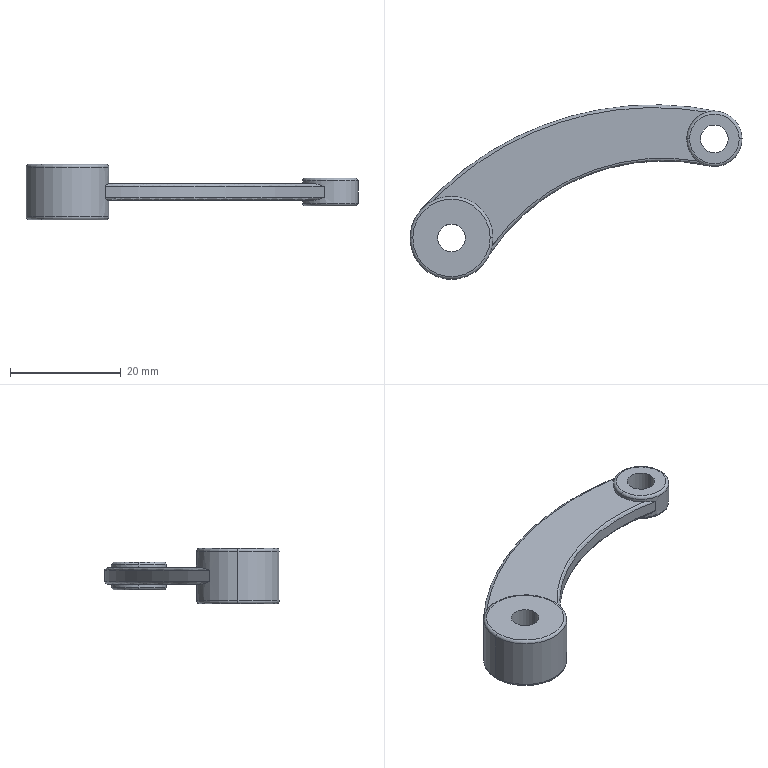Part | SolidWorks | features Fillet 2, ICE 2, Extrusion 1, MirrorPattern 1 | 1 solid | 28 faces | box 60.037 x 31.564 x 10 mm | volume 3346 mm3 | torus 12 | cylinder 10 | plane 6 | commonest cylinder face diameters 5 x4 10 x2 15 x2 75.265 x1 112.752 x1
STEP:
#1=CARTESIAN_POINT('',(-7.5,0.,4.5));
#2=VERTEX_POINT('',#1);
#3=CARTESIAN_POINT('',(7.5,0.,4.5));
#4=VERTEX_POINT('',#3);
#5=CARTESIAN_POINT('',(0.,0.,4.5));
#6=DIRECTION('',(0.,0.,-1.));
#7=DIRECTION('',(1.,0.,0.));
#8=AXIS2_PLACEMENT_3D('',#5,#6,#7);
#9=CIRCLE('',#8,7.5);
#10=EDGE_CURVE('',#2,#4,#9,.T.);
#11=ORIENTED_EDGE('',*,*,#10,.F.);
#12=CARTESIAN_POINT('',(-7.,0.,5.));
#13=VERTEX_POINT('',#12);
#14=CARTESIAN_POINT('',(-7.,0.,4.5));
#15=DIRECTION('',(0.,1.,0.));
#16=DIRECTION('',(-1.,0.,0.));
#17=AXIS2_PLACEMENT_3D('',#14,#15,#16);
#18=CIRCLE('',#17,0.5);
#19=EDGE_CURVE('',#2,#13,#18,.T.);
#20=ORIENTED_EDGE('',*,*,#19,.T.);
#21=CARTESIAN_POINT('',(7.,0.,5.));
#22=VERTEX_POINT('',#21);
#23=CARTESIAN_POINT('',(0.,0.,5.));
#24=DIRECTION('',(0.,0.,1.));
#25=DIRECTION('',(1.,0.,0.));
#26=AXIS2_PLACEMENT_3D('',#23,#24,#25);
#27=CIRCLE('',#26,7.);
#28=EDGE_CURVE('',#22,#13,#27,.T.);
#29=ORIENTED_EDGE('',*,*,#28,.F.);
#30=CARTESIAN_POINT('',(7.,0.,4.5));
#31=DIRECTION('',(0.,-1.,0.));
#32=DIRECTION('',(0.,0.,-1.));
#33=AXIS2_PLACEMENT_3D('',#30,#31,#32);
#34=CIRCLE('',#33,0.5);
#35=EDGE_CURVE('',#4,#22,#34,.T.);
#36=ORIENTED_EDGE('',*,*,#35,.F.);
#37=EDGE_LOOP('',(#11,#20,#29,#36));
#38=FACE_OUTER_BOUND('',#37,.T.);
#39=CARTESIAN_POINT('',(0.,0.,4.5));
#40=DIRECTION('',(0.,0.,1.));
#41=DIRECTION('',(1.,0.,0.));
#42=AXIS2_PLACEMENT_3D('',#39,#40,#41);
#43=TOROIDAL_SURFACE('',#42,7.,0.5);
#44=ADVANCED_FACE('',(#38),#43,.T.);
#45=CARTESIAN_POINT('',(42.537,17.903,2.));
#46=VERTEX_POINT('',#45);
#47=CARTESIAN_POINT('',(52.537,17.903,2.));
#48=VERTEX_POINT('',#47);
#49=CARTESIAN_POINT('',(47.537,17.903,2.));
#50=DIRECTION('',(0.,0.,-1.));
#51=DIRECTION('',(1.,0.,0.));
#52=AXIS2_PLACEMENT_3D('',#49,#50,#51);
#53=CIRCLE('',#52,5.);
#54=EDGE_CURVE('',#46,#48,#53,.T.);
#55=ORIENTED_EDGE('',*,*,#54,.F.);
#56=CARTESIAN_POINT('',(43.037,17.903,2.5));
#57=VERTEX_POINT('',#56);
#58=CARTESIAN_POINT('',(43.037,17.903,2.));
#59=DIRECTION('',(0.,1.,0.));
#60=DIRECTION('',(-1.,0.,0.));
#61=AXIS2_PLACEMENT_3D('',#58,#59,#60);
#62=CIRCLE('',#61,0.5);
#63=EDGE_CURVE('',#46,#57,#62,.T.);
#64=ORIENTED_EDGE('',*,*,#63,.T.);
#65=CARTESIAN_POINT('',(52.037,17.903,2.5));
#66=VERTEX_POINT('',#65);
#67=CARTESIAN_POINT('',(47.537,17.903,2.5));
#68=DIRECTION('',(0.,0.,1.));
#69=DIRECTION('',(1.,0.,0.));
#70=AXIS2_PLACEMENT_3D('',#67,#68,#69);
#71=CIRCLE('',#70,4.5);
#72=EDGE_CURVE('',#66,#57,#71,.T.);
#73=ORIENTED_EDGE('',*,*,#72,.F.);
#74=CARTESIAN_POINT('',(52.037,17.903,2.));
#75=DIRECTION('',(0.,-1.,0.));
#76=DIRECTION('',(0.,0.,-1.));
#77=AXIS2_PLACEMENT_3D('',#74,#75,#76);
#78=CIRCLE('',#77,0.5);
#79=EDGE_CURVE('',#48,#66,#78,.T.);
#80=ORIENTED_EDGE('',*,*,#79,.F.);
#81=EDGE_LOOP('',(#55,#64,#73,#80));
#82=FACE_OUTER_BOUND('',#81,.T.);
#83=CARTESIAN_POINT('',(47.537,17.903,2.));
#84=DIRECTION('',(0.,0.,1.));
#85=DIRECTION('',(1.,0.,0.));
#86=AXIS2_PLACEMENT_3D('',#83,#84,#85);
#87=TOROIDAL_SURFACE('',#86,4.5,0.5);
#88=ADVANCED_FACE('',(#82),#87,.T.);
#89=CARTESIAN_POINT('',(52.537,17.903,-2.));
#90=VERTEX_POINT('',#89);
#91=CARTESIAN_POINT('',(42.537,17.903,-2.));
#92=VERTEX_POINT('',#91);
#93=CARTESIAN_POINT('',(47.537,17.903,-2.));
#94=DIRECTION('',(0.,0.,1.));
#95=DIRECTION('',(-1.,0.,0.));
#96=AXIS2_PLACEMENT_3D('',#93,#94,#95);
#97=CIRCLE('',#96,5.);
#98=EDGE_CURVE('',#90,#92,#97,.T.);
#99=ORIENTED_EDGE('',*,*,#98,.F.);
#100=CARTESIAN_POINT('',(52.037,17.903,-2.5));
#101=VERTEX_POINT('',#100);
#102=CARTESIAN_POINT('',(52.037,17.903,-2.));
#103=DIRECTION('',(0.,1.,0.));
#104=DIRECTION('',(-1.,0.,0.));
#105=AXIS2_PLACEMENT_3D('',#102,#103,#104);
#106=CIRCLE('',#105,0.5);
#107=EDGE_CURVE('',#90,#101,#106,.T.);
#108=ORIENTED_EDGE('',*,*,#107,.T.);
#109=CARTESIAN_POINT('',(43.037,17.903,-2.5));
#110=VERTEX_POINT('',#109);
#111=CARTESIAN_POINT('',(47.537,17.903,-2.5));
#112=DIRECTION('',(0.,0.,-1.));
#113=DIRECTION('',(-1.,0.,0.));
#114=AXIS2_PLACEMENT_3D('',#111,#112,#113);
#115=CIRCLE('',#114,4.5);
#116=EDGE_CURVE('',#110,#101,#115,.T.);
#117=ORIENTED_EDGE('',*,*,#116,.F.);
#118=CARTESIAN_POINT('',(43.037,17.903,-2.));
#119=DIRECTION('',(0.,-1.,0.));
#120=DIRECTION('',(0.,0.,-1.));
#121=AXIS2_PLACEMENT_3D('',#118,#119,#120);
#122=CIRCLE('',#121,0.5);
#123=EDGE_CURVE('',#92,#110,#122,.T.);
#124=ORIENTED_EDGE('',*,*,#123,.F.);
#125=EDGE_LOOP('',(#99,#108,#117,#124));
#126=FACE_OUTER_BOUND('',#125,.T.);
#127=CARTESIAN_POINT('',(47.537,17.903,-2.));
#128=DIRECTION('',(0.,0.,-1.));
#129=DIRECTION('',(-1.,0.,0.));
#130=AXIS2_PLACEMENT_3D('',#127,#128,#129);
#131=TOROIDAL_SURFACE('',#130,4.5,0.5);
#132=ADVANCED_FACE('',(#126),#131,.T.);
#133=CARTESIAN_POINT('',(-7.,0.,-5.));
#134=VERTEX_POINT('',#133);
#135=CARTESIAN_POINT('',(7.,0.,-5.));
#136=VERTEX_POINT('',#135);
#137=CARTESIAN_POINT('',(0.,0.,-5.));
#138=DIRECTION('',(0.,0.,-1.));
#139=DIRECTION('',(1.,0.,0.));
#140=AXIS2_PLACEMENT_3D('',#137,#138,#139);
#141=CIRCLE('',#140,7.);
#142=EDGE_CURVE('',#134,#136,#141,.T.);
#143=ORIENTED_EDGE('',*,*,#142,.F.);
#144=CARTESIAN_POINT('',(-7.5,0.,-4.5));
#145=VERTEX_POINT('',#144);
#146=CARTESIAN_POINT('',(-7.,0.,-4.5));
#147=DIRECTION('',(0.,1.,0.));
#148=DIRECTION('',(-1.,0.,0.));
#149=AXIS2_PLACEMENT_3D('',#146,#147,#148);
#150=CIRCLE('',#149,0.5);
#151=EDGE_CURVE('',#134,#145,#150,.T.);
#152=ORIENTED_EDGE('',*,*,#151,.T.);
#153=CARTESIAN_POINT('',(7.5,0.,-4.5));
#154=VERTEX_POINT('',#153);
#155=CARTESIAN_POINT('',(0.,0.,-4.5));
#156=DIRECTION('',(0.,0.,1.));
#157=DIRECTION('',(1.,0.,0.));
#158=AXIS2_PLACEMENT_3D('',#155,#156,#157);
#159=CIRCLE('',#158,7.5);
#160=EDGE_CURVE('',#154,#145,#159,.T.);
#161=ORIENTED_EDGE('',*,*,#160,.F.);
#162=CARTESIAN_POINT('',(7.,0.,-4.5));
#163=DIRECTION('',(0.,-1.,0.));
#164=DIRECTION('',(0.,0.,-1.));
#165=AXIS2_PLACEMENT_3D('',#162,#163,#164);
#166=CIRCLE('',#165,0.5);
#167=EDGE_CURVE('',#136,#154,#166,.T.);
#168=ORIENTED_EDGE('',*,*,#167,.F.);
#169=EDGE_LOOP('',(#143,#152,#161,#168));
#170=FACE_OUTER_BOUND('',#169,.T.);
#171=CARTESIAN_POINT('',(0.,0.,-4.5));
#172=DIRECTION('',(0.,0.,1.));
#173=DIRECTION('',(1.,0.,0.));
#174=AXIS2_PLACEMENT_3D('',#171,#172,#173);
#175=TOROIDAL_SURFACE('',#174,7.,0.5);
#176=ADVANCED_FACE('',(#170),#175,.T.);
#177=CARTESIAN_POINT('',(45.037,17.903,2.5));
#178=VERTEX_POINT('',#177);
#179=CARTESIAN_POINT('',(50.037,17.903,2.5));
#180=VERTEX_POINT('',#179);
#181=CARTESIAN_POINT('',(47.537,17.903,2.5));
#182=DIRECTION('',(0.,0.,1.));
#183=DIRECTION('',(1.,0.,0.));
#184=AXIS2_PLACEMENT_3D('',#181,#182,#183);
#185=CIRCLE('',#184,2.5);
#186=EDGE_CURVE('',#178,#180,#185,.T.);
#187=ORIENTED_EDGE('',*,*,#186,.T.);
#188=CARTESIAN_POINT('',(50.037,17.903,-2.5));
#189=VERTEX_POINT('',#188);
#190=CARTESIAN_POINT('',(50.037,17.903,1.5));
#191=DIRECTION('',(0.,0.,-1.));
#192=VECTOR('',#191,1000.);
#193=LINE('',#190,#192);
#194=EDGE_CURVE('',#180,#189,#193,.T.);
#195=ORIENTED_EDGE('',*,*,#194,.T.);
#196=CARTESIAN_POINT('',(45.037,17.903,-2.5));
#197=VERTEX_POINT('',#196);
#198=CARTESIAN_POINT('',(47.537,17.903,-2.5));
#199=DIRECTION('',(0.,0.,1.));
#200=DIRECTION('',(1.,0.,0.));
#201=AXIS2_PLACEMENT_3D('',#198,#199,#200);
#202=CIRCLE('',#201,2.5);
#203=EDGE_CURVE('',#197,#189,#202,.T.);
#204=ORIENTED_EDGE('',*,*,#203,.F.);
#205=CARTESIAN_POINT('',(45.037,17.903,1.5));
#206=DIRECTION('',(0.,0.,-1.));
#207=VECTOR('',#206,1000.);
#208=LINE('',#205,#207);
#209=EDGE_CURVE('',#178,#197,#208,.T.);
#210=ORIENTED_EDGE('',*,*,#209,.F.);
#211=EDGE_LOOP('',(#187,#195,#204,#210));
#212=FACE_OUTER_BOUND('',#211,.T.);
#213=CARTESIAN_POINT('',(47.537,17.903,1.5));
#214=DIRECTION('',(0.,0.,-1.));
#215=DIRECTION('',(-1.,0.,0.));
#216=AXIS2_PLACEMENT_3D('',#213,#214,#215);
#217=CYLINDRICAL_SURFACE('',#216,2.5);
#218=ADVANCED_FACE('',(#212),#217,.F.);
#219=ORIENTED_EDGE('',*,*,#54,.T.);
#220=CARTESIAN_POINT('',(52.537,17.903,1.5));
#221=DIRECTION('',(0.,0.,-1.));
#222=VECTOR('',#221,1000.);
#223=LINE('',#220,#222);
#224=EDGE_CURVE('',#48,#90,#223,.T.);
#225=ORIENTED_EDGE('',*,*,#224,.T.);
#226=ORIENTED_EDGE('',*,*,#98,.T.);
#227=CARTESIAN_POINT('',(42.537,17.903,-1.5));
#228=VERTEX_POINT('',#227);
#229=CARTESIAN_POINT('',(42.537,17.903,1.5));
#230=DIRECTION('',(0.,0.,-1.));
#231=VECTOR('',#230,1000.);
#232=LINE('',#229,#231);
#233=EDGE_CURVE('',#228,#92,#232,.T.);
#234=ORIENTED_EDGE('',*,*,#233,.F.);
#235=CARTESIAN_POINT('',(46.257,22.736,-1.5));
#236=VERTEX_POINT('',#235);
#237=CARTESIAN_POINT('',(47.537,17.903,-1.5));
#238=DIRECTION('',(0.,0.,1.));
#239=DIRECTION('',(1.,0.,0.));
#240=AXIS2_PLACEMENT_3D('',#237,#238,#239);
#241=CIRCLE('',#240,5.);
#242=EDGE_CURVE('',#236,#228,#241,.T.);
#243=ORIENTED_EDGE('',*,*,#242,.F.);
#244=CARTESIAN_POINT('',(48.594,22.79,-1.));
#245=VERTEX_POINT('',#244);
#246=CARTESIAN_POINT('',(46.257,22.736,-1.5));
#247=CARTESIAN_POINT('',(46.454,22.788,-1.5));
#248=CARTESIAN_POINT('',(46.651,22.828,-1.479));
#249=CARTESIAN_POINT('',(47.045,22.882,-1.418));
#250=CARTESIAN_POINT('',(47.243,22.898,-1.376));
#251=CARTESIAN_POINT('',(47.635,22.906,-1.281));
#252=CARTESIAN_POINT('',(47.829,22.898,-1.228));
#253=CARTESIAN_POINT('',(48.214,22.86,-1.117));
#254=CARTESIAN_POINT('',(48.406,22.83,-1.058));
#255=CARTESIAN_POINT('',(48.594,22.79,-1.));
#256=B_SPLINE_CURVE_WITH_KNOTS('',3,(#246,#247,#248,#249,#250,#251,#252,#253,#254,#255),.UNSPECIFIED.,.F.,.F.,(4,2,2,2,4),(0.,0.0006033,0.001207,0.00181,0.002413),.UNSPECIFIED.);
#257=EDGE_CURVE('',#236,#245,#256,.T.);
#258=ORIENTED_EDGE('',*,*,#257,.T.);
#259=CARTESIAN_POINT('',(48.594,22.79,1.));
#260=VERTEX_POINT('',#259);
#261=CARTESIAN_POINT('',(48.594,22.79,1.5));
#262=DIRECTION('',(0.,0.,-1.));
#263=VECTOR('',#262,1000.);
#264=LINE('',#261,#263);
#265=EDGE_CURVE('',#260,#245,#264,.T.);
#266=ORIENTED_EDGE('',*,*,#265,.F.);
#267=CARTESIAN_POINT('',(46.257,22.736,1.5));
#268=VERTEX_POINT('',#267);
#269=CARTESIAN_POINT('',(48.594,22.79,1.));
#270=CARTESIAN_POINT('',(48.406,22.83,1.058));
#271=CARTESIAN_POINT('',(48.214,22.86,1.117));
#272=CARTESIAN_POINT('',(47.829,22.898,1.228));
#273=CARTESIAN_POINT('',(47.635,22.906,1.281));
#274=CARTESIAN_POINT('',(47.243,22.898,1.376));
#275=CARTESIAN_POINT('',(47.045,22.882,1.418));
#276=CARTESIAN_POINT('',(46.651,22.828,1.479));
#277=CARTESIAN_POINT('',(46.454,22.788,1.5));
#278=CARTESIAN_POINT('',(46.257,22.736,1.5));
#279=B_SPLINE_CURVE_WITH_KNOTS('',3,(#269,#270,#271,#272,#273,#274,#275,#276,#277,#278),.UNSPECIFIED.,.F.,.F.,(4,2,2,2,4),(-0.00001481,0.0005878,0.00119,0.001793,0.002396),.UNSPECIFIED.);
#280=EDGE_CURVE('',#260,#268,#279,.T.);
#281=ORIENTED_EDGE('',*,*,#280,.T.);
#282=CARTESIAN_POINT('',(42.537,17.903,1.5));
#283=VERTEX_POINT('',#282);
#284=CARTESIAN_POINT('',(47.537,17.903,1.5));
#285=DIRECTION('',(0.,0.,1.));
#286=DIRECTION('',(1.,0.,0.));
#287=AXIS2_PLACEMENT_3D('',#284,#285,#286);
#288=CIRCLE('',#287,5.);
#289=EDGE_CURVE('',#268,#283,#288,.T.);
#290=ORIENTED_EDGE('',*,*,#289,.T.);
#291=CARTESIAN_POINT('',(42.537,17.903,1.5));
#292=DIRECTION('',(0.,0.,-1.));
#293=VECTOR('',#292,1000.);
#294=LINE('',#291,#293);
#295=EDGE_CURVE('',#46,#283,#294,.T.);
#296=ORIENTED_EDGE('',*,*,#295,.F.);
#297=EDGE_LOOP('',(#219,#225,#226,#234,#243,#258,#266,#281,#290,#296));
#298=FACE_OUTER_BOUND('',#297,.T.);
#299=CARTESIAN_POINT('',(47.537,17.903,1.5));
#300=DIRECTION('',(0.,0.,-1.));
#301=DIRECTION('',(-1.,0.,0.));
#302=AXIS2_PLACEMENT_3D('',#299,#300,#301);
#303=CYLINDRICAL_SURFACE('',#302,5.);
#304=ADVANCED_FACE('',(#298),#303,.T.);
#305=CARTESIAN_POINT('',(-2.5,0.,5.));
#306=VERTEX_POINT('',#305);
#307=CARTESIAN_POINT('',(2.5,0.,5.));
#308=VERTEX_POINT('',#307);
#309=CARTESIAN_POINT('',(0.,0.,5.));
#310=DIRECTION('',(0.,0.,1.));
#311=DIRECTION('',(1.,0.,0.));
#312=AXIS2_PLACEMENT_3D('',#309,#310,#311);
#313=CIRCLE('',#312,2.5);
#314=EDGE_CURVE('',#306,#308,#313,.T.);
#315=ORIENTED_EDGE('',*,*,#314,.T.);
#316=CARTESIAN_POINT('',(2.5,0.,-5.));
#317=VERTEX_POINT('',#316);
#318=CARTESIAN_POINT('',(2.5,0.,5.));
#319=DIRECTION('',(0.,0.,-1.));
#320=VECTOR('',#319,1000.);
#321=LINE('',#318,#320);
#322=EDGE_CURVE('',#308,#317,#321,.T.);
#323=ORIENTED_EDGE('',*,*,#322,.T.);
#324=CARTESIAN_POINT('',(-2.5,0.,-5.));
#325=VERTEX_POINT('',#324);
#326=CARTESIAN_POINT('',(0.,0.,-5.));
#327=DIRECTION('',(0.,0.,1.));
#328=DIRECTION('',(1.,0.,0.));
#329=AXIS2_PLACEMENT_3D('',#326,#327,#328);
#330=CIRCLE('',#329,2.5);
#331=EDGE_CURVE('',#325,#317,#330,.T.);
#332=ORIENTED_EDGE('',*,*,#331,.F.);
#333=CARTESIAN_POINT('',(-2.5,0.,5.));
#334=DIRECTION('',(0.,0.,-1.));
#335=VECTOR('',#334,1000.);
#336=LINE('',#333,#335);
#337=EDGE_CURVE('',#306,#325,#336,.T.);
#338=ORIENTED_EDGE('',*,*,#337,.F.);
#339=EDGE_LOOP('',(#315,#323,#332,#338));
#340=FACE_OUTER_BOUND('',#339,.T.);
#341=CARTESIAN_POINT('',(0.,0.,5.));
#342=DIRECTION('',(0.,0.,-1.));
#343=DIRECTION('',(-1.,0.,0.));
#344=AXIS2_PLACEMENT_3D('',#341,#342,#343);
#345=CYLINDRICAL_SURFACE('',#344,2.5);
#346=ADVANCED_FACE('',(#340),#345,.F.);
#347=ORIENTED_EDGE('',*,*,#10,.T.);
#348=CARTESIAN_POINT('',(7.5,0.,1.5));
#349=VERTEX_POINT('',#348);
#350=CARTESIAN_POINT('',(7.5,0.,5.));
#351=DIRECTION('',(0.,0.,-1.));
#352=VECTOR('',#351,1000.);
#353=LINE('',#350,#352);
#354=EDGE_CURVE('',#4,#349,#353,.T.);
#355=ORIENTED_EDGE('',*,*,#354,.T.);
#356=CARTESIAN_POINT('',(-3.29,6.74,1.5));
#357=VERTEX_POINT('',#356);
#358=CARTESIAN_POINT('',(0.,0.,1.5));
#359=DIRECTION('',(0.,0.,-1.));
#360=DIRECTION('',(1.,0.,0.));
#361=AXIS2_PLACEMENT_3D('',#358,#359,#360);
#362=CIRCLE('',#361,7.5);
#363=EDGE_CURVE('',#357,#349,#362,.T.);
#364=ORIENTED_EDGE('',*,*,#363,.F.);
#365=CARTESIAN_POINT('',(-5.52,5.078,1.));
#366=VERTEX_POINT('',#365);
#367=CARTESIAN_POINT('',(-3.29,6.74,1.5));
#368=CARTESIAN_POINT('',(-3.505,6.635,1.5));
#369=CARTESIAN_POINT('',(-3.712,6.521,1.482));
#370=CARTESIAN_POINT('',(-4.114,6.275,1.425));
#371=CARTESIAN_POINT('',(-4.309,6.143,1.387));
#372=CARTESIAN_POINT('',(-4.684,5.862,1.298));
#373=CARTESIAN_POINT('',(-4.864,5.714,1.248));
#374=CARTESIAN_POINT('',(-5.122,5.48,1.168));
#375=CARTESIAN_POINT('',(-5.206,5.4,1.141));
#376=CARTESIAN_POINT('',(-5.329,5.278,1.098));
#377=CARTESIAN_POINT('',(-5.369,5.237,1.083));
#378=CARTESIAN_POINT('',(-5.429,5.175,1.059));
#379=CARTESIAN_POINT('',(-5.449,5.154,1.051));
#380=CARTESIAN_POINT('',(-5.478,5.123,1.037));
#381=CARTESIAN_POINT('',(-5.487,5.113,1.032));
#382=CARTESIAN_POINT('',(-5.501,5.098,1.023));
#383=CARTESIAN_POINT('',(-5.506,5.093,1.02));
#384=CARTESIAN_POINT('',(-5.515,5.083,1.013));
#385=CARTESIAN_POINT('',(-5.52,5.078,1.008));
#386=CARTESIAN_POINT('',(-5.52,5.078,1.));
#387=B_SPLINE_CURVE_WITH_KNOTS('',3,(#367,#368,#369,#370,#371,#372,#373,#374,#375,#376,#377,#378,#379,#380,#381,#382,#383,#384,#385,#386),.UNSPECIFIED.,.F.,.F.,(4,2,2,2,2,2,2,2,2,4),(0.,0.0007118,0.001424,0.002135,0.002491,0.002669,0.002758,0.002803,0.002825,0.002847),.UNSPECIFIED.);
#388=EDGE_CURVE('',#357,#366,#387,.T.);
#389=ORIENTED_EDGE('',*,*,#388,.T.);
#390=CARTESIAN_POINT('',(-5.52,5.078,-1.));
#391=VERTEX_POINT('',#390);
#392=CARTESIAN_POINT('',(-5.52,5.078,1.5));
#393=DIRECTION('',(0.,0.,-1.));
#394=VECTOR('',#393,1000.);
#395=LINE('',#392,#394);
#396=EDGE_CURVE('',#366,#391,#395,.T.);
#397=ORIENTED_EDGE('',*,*,#396,.T.);
#398=CARTESIAN_POINT('',(-3.29,6.74,-1.5));
#399=VERTEX_POINT('',#398);
#400=CARTESIAN_POINT('',(-5.52,5.078,-1.));
#401=CARTESIAN_POINT('',(-5.52,5.078,-1.008));
#402=CARTESIAN_POINT('',(-5.514,5.083,-1.013));
#403=CARTESIAN_POINT('',(-5.506,5.093,-1.02));
#404=CARTESIAN_POINT('',(-5.501,5.098,-1.024));
#405=CARTESIAN_POINT('',(-5.487,5.113,-1.032));
#406=CARTESIAN_POINT('',(-5.477,5.123,-1.037));
#407=CARTESIAN_POINT('',(-5.448,5.154,-1.051));
#408=CARTESIAN_POINT('',(-5.428,5.175,-1.059));
#409=CARTESIAN_POINT('',(-5.369,5.238,-1.083));
#410=CARTESIAN_POINT('',(-5.328,5.279,-1.098));
#411=CARTESIAN_POINT('',(-5.205,5.401,-1.141));
#412=CARTESIAN_POINT('',(-5.12,5.481,-1.169));
#413=CARTESIAN_POINT('',(-4.861,5.716,-1.249));
#414=CARTESIAN_POINT('',(-4.681,5.865,-1.299));
#415=CARTESIAN_POINT('',(-4.308,6.144,-1.387));
#416=CARTESIAN_POINT('',(-4.114,6.275,-1.425));
#417=CARTESIAN_POINT('',(-3.714,6.52,-1.481));
#418=CARTESIAN_POINT('',(-3.506,6.634,-1.5));
#419=CARTESIAN_POINT('',(-3.29,6.74,-1.5));
#420=B_SPLINE_CURVE_WITH_KNOTS('',3,(#400,#401,#402,#403,#404,#405,#406,#407,#408,#409,#410,#411,#412,#413,#414,#415,#416,#417,#418,#419),.UNSPECIFIED.,.F.,.F.,(4,2,2,2,2,2,2,2,2,4),(0.,0.00002266,0.00004532,0.00009064,0.0001813,0.0003626,0.0007252,0.00145,0.002175,0.002901),.UNSPECIFIED.);
#421=EDGE_CURVE('',#391,#399,#420,.T.);
#422=ORIENTED_EDGE('',*,*,#421,.T.);
#423=CARTESIAN_POINT('',(7.5,0.,-1.5));
#424=VERTEX_POINT('',#423);
#425=CARTESIAN_POINT('',(0.,0.,-1.5));
#426=DIRECTION('',(0.,0.,-1.));
#427=DIRECTION('',(1.,0.,0.));
#428=AXIS2_PLACEMENT_3D('',#425,#426,#427);
#429=CIRCLE('',#428,7.5);
#430=EDGE_CURVE('',#399,#424,#429,.T.);
#431=ORIENTED_EDGE('',*,*,#430,.T.);
#432=CARTESIAN_POINT('',(7.5,0.,5.));
#433=DIRECTION('',(0.,0.,-1.));
#434=VECTOR('',#433,1000.);
#435=LINE('',#432,#434);
#436=EDGE_CURVE('',#424,#154,#435,.T.);
#437=ORIENTED_EDGE('',*,*,#436,.T.);
#438=ORIENTED_EDGE('',*,*,#160,.T.);
#439=CARTESIAN_POINT('',(-7.5,0.,5.));
#440=DIRECTION('',(0.,0.,-1.));
#441=VECTOR('',#440,1000.);
#442=LINE('',#439,#441);
#443=EDGE_CURVE('',#2,#145,#442,.T.);
#444=ORIENTED_EDGE('',*,*,#443,.F.);
#445=EDGE_LOOP('',(#347,#355,#364,#389,#397,#422,#431,#437,#438,#444));
#446=FACE_OUTER_BOUND('',#445,.T.);
#447=CARTESIAN_POINT('',(0.,0.,5.));
#448=DIRECTION('',(0.,0.,-1.));
#449=DIRECTION('',(-1.,0.,0.));
#450=AXIS2_PLACEMENT_3D('',#447,#448,#449);
#451=CYLINDRICAL_SURFACE('',#450,7.5);
#452=ADVANCED_FACE('',(#446),#451,.T.);
#453=ORIENTED_EDGE('',*,*,#289,.F.);
#454=CARTESIAN_POINT('',(36.674,-32.312,1.5));
#455=DIRECTION('',(0.,0.,1.));
#456=DIRECTION('',(-1.,0.,0.));
#457=AXIS2_PLACEMENT_3D('',#454,#455,#456);
#458=CIRCLE('',#457,55.876);
#459=EDGE_CURVE('',#268,#357,#458,.T.);
#460=ORIENTED_EDGE('',*,*,#459,.T.);
#461=ORIENTED_EDGE('',*,*,#363,.T.);
#462=CARTESIAN_POINT('',(7.37,-1.392,1.5));
#463=VERTEX_POINT('',#462);
#464=CARTESIAN_POINT('',(0.,0.,1.5));
#465=DIRECTION('',(0.,0.,-1.));
#466=DIRECTION('',(1.,0.,0.));
#467=AXIS2_PLACEMENT_3D('',#464,#465,#466);
#468=CIRCLE('',#467,7.5);
#469=EDGE_CURVE('',#349,#463,#468,.T.);
#470=ORIENTED_EDGE('',*,*,#469,.T.);
#471=CARTESIAN_POINT('',(44.537,13.903,1.5));
#472=VERTEX_POINT('',#471);
#473=CARTESIAN_POINT('',(38.286,-23.714,1.5));
#474=DIRECTION('',(0.,0.,-1.));
#475=DIRECTION('',(-1.,0.,0.));
#476=AXIS2_PLACEMENT_3D('',#473,#474,#475);
#477=CIRCLE('',#476,38.132);
#478=EDGE_CURVE('',#463,#472,#477,.T.);
#479=ORIENTED_EDGE('',*,*,#478,.T.);
#480=CARTESIAN_POINT('',(47.537,17.903,1.5));
#481=DIRECTION('',(0.,0.,1.));
#482=DIRECTION('',(1.,0.,0.));
#483=AXIS2_PLACEMENT_3D('',#480,#481,#482);
#484=CIRCLE('',#483,5.);
#485=EDGE_CURVE('',#283,#472,#484,.T.);
#486=ORIENTED_EDGE('',*,*,#485,.F.);
#487=EDGE_LOOP('',(#453,#460,#461,#470,#479,#486));
#488=FACE_OUTER_BOUND('',#487,.T.);
#489=CARTESIAN_POINT('',(42.911,-2.906,1.5));
#490=DIRECTION('',(0.,0.,-1.));
#491=DIRECTION('',(-1.,0.,0.));
#492=AXIS2_PLACEMENT_3D('',#489,#490,#491);
#493=PLANE('',#492);
#494=ADVANCED_FACE('',(#488),#493,.F.);
#495=ORIENTED_EDGE('',*,*,#354,.F.);
#496=CARTESIAN_POINT('',(0.,0.,4.5));
#497=DIRECTION('',(0.,0.,-1.));
#498=DIRECTION('',(1.,0.,0.));
#499=AXIS2_PLACEMENT_3D('',#496,#497,#498);
#500=CIRCLE('',#499,7.5);
#501=EDGE_CURVE('',#4,#2,#500,.T.);
#502=ORIENTED_EDGE('',*,*,#501,.T.);
#503=ORIENTED_EDGE('',*,*,#443,.T.);
#504=CARTESIAN_POINT('',(0.,0.,-4.5));
#505=DIRECTION('',(0.,0.,1.));
#506=DIRECTION('',(1.,0.,0.));
#507=AXIS2_PLACEMENT_3D('',#504,#505,#506);
#508=CIRCLE('',#507,7.5);
#509=EDGE_CURVE('',#145,#154,#508,.T.);
#510=ORIENTED_EDGE('',*,*,#509,.T.);
#511=ORIENTED_EDGE('',*,*,#436,.F.);
#512=CARTESIAN_POINT('',(7.37,-1.392,-1.5));
#513=VERTEX_POINT('',#512);
#514=CARTESIAN_POINT('',(0.,0.,-1.5));
#515=DIRECTION('',(0.,0.,-1.));
#516=DIRECTION('',(1.,0.,0.));
#517=AXIS2_PLACEMENT_3D('',#514,#515,#516);
#518=CIRCLE('',#517,7.5);
#519=EDGE_CURVE('',#424,#513,#518,.T.);
#520=ORIENTED_EDGE('',*,*,#519,.T.);
#521=CARTESIAN_POINT('',(6.886,-2.972,-1.));
#522=VERTEX_POINT('',#521);
#523=CARTESIAN_POINT('',(7.37,-1.392,-1.5));
#524=CARTESIAN_POINT('',(7.314,-1.687,-1.5));
#525=CARTESIAN_POINT('',(7.242,-1.971,-1.456));
#526=CARTESIAN_POINT('',(7.112,-2.385,-1.351));
#527=CARTESIAN_POINT('',(7.065,-2.521,-1.309));
#528=CARTESIAN_POINT('',(6.991,-2.716,-1.228));
#529=CARTESIAN_POINT('',(6.966,-2.78,-1.199));
#530=CARTESIAN_POINT('',(6.929,-2.87,-1.142));
#531=CARTESIAN_POINT('',(6.917,-2.899,-1.122));
#532=CARTESIAN_POINT('',(6.896,-2.949,-1.07));
#533=CARTESIAN_POINT('',(6.886,-2.972,-1.038));
#534=CARTESIAN_POINT('',(6.886,-2.972,-1.));
#535=B_SPLINE_CURVE_WITH_KNOTS('',3,(#523,#524,#525,#526,#527,#528,#529,#530,#531,#532,#533,#534),.UNSPECIFIED.,.F.,.F.,(4,2,2,2,2,4),(0.,0.0008878,0.001332,0.001554,0.001665,0.001776),.UNSPECIFIED.);
#536=EDGE_CURVE('',#513,#522,#535,.T.);
#537=ORIENTED_EDGE('',*,*,#536,.T.);
#538=CARTESIAN_POINT('',(6.886,-2.972,1.));
#539=VERTEX_POINT('',#538);
#540=CARTESIAN_POINT('',(6.886,-2.972,1.5));
#541=DIRECTION('',(0.,0.,-1.));
#542=VECTOR('',#541,1000.);
#543=LINE('',#540,#542);
#544=EDGE_CURVE('',#539,#522,#543,.T.);
#545=ORIENTED_EDGE('',*,*,#544,.F.);
#546=CARTESIAN_POINT('',(6.886,-2.972,1.));
#547=CARTESIAN_POINT('',(6.886,-2.972,1.038));
#548=CARTESIAN_POINT('',(6.896,-2.949,1.071));
#549=CARTESIAN_POINT('',(6.918,-2.898,1.122));
#550=CARTESIAN_POINT('',(6.93,-2.869,1.143));
#551=CARTESIAN_POINT('',(6.967,-2.779,1.199));
#552=CARTESIAN_POINT('',(6.992,-2.715,1.229));
#553=CARTESIAN_POINT('',(7.066,-2.519,1.31));
#554=CARTESIAN_POINT('',(7.112,-2.384,1.351));
#555=CARTESIAN_POINT('',(7.199,-2.11,1.421));
#556=CARTESIAN_POINT('',(7.238,-1.97,1.449));
#557=CARTESIAN_POINT('',(7.31,-1.686,1.488));
#558=CARTESIAN_POINT('',(7.342,-1.54,1.5));
#559=CARTESIAN_POINT('',(7.37,-1.392,1.5));
#560=B_SPLINE_CURVE_WITH_KNOTS('',3,(#546,#547,#548,#549,#550,#551,#552,#553,#554,#555,#556,#557,#558,#559),.UNSPECIFIED.,.F.,.F.,(4,2,2,2,2,2,4),(0.,0.0001131,0.0002262,0.0004523,0.0009046,0.001357,0.001809),.UNSPECIFIED.);
#561=EDGE_CURVE('',#539,#463,#560,.T.);
#562=ORIENTED_EDGE('',*,*,#561,.T.);
#563=ORIENTED_EDGE('',*,*,#469,.F.);
#564=EDGE_LOOP('',(#495,#502,#503,#510,#511,#520,#537,#545,#562,#563));
#565=FACE_OUTER_BOUND('',#564,.T.);
#566=CARTESIAN_POINT('',(0.,0.,5.));
#567=DIRECTION('',(0.,0.,-1.));
#568=DIRECTION('',(-1.,0.,0.));
#569=AXIS2_PLACEMENT_3D('',#566,#567,#568);
#570=CYLINDRICAL_SURFACE('',#569,7.5);
#571=ADVANCED_FACE('',(#565),#570,.T.);
#572=ORIENTED_EDGE('',*,*,#28,.T.);
#573=CARTESIAN_POINT('',(0.,0.,5.));
#574=DIRECTION('',(0.,0.,1.));
#575=DIRECTION('',(1.,0.,0.));
#576=AXIS2_PLACEMENT_3D('',#573,#574,#575);
#577=CIRCLE('',#576,7.);
#578=EDGE_CURVE('',#13,#22,#577,.T.);
#579=ORIENTED_EDGE('',*,*,#578,.T.);
#580=EDGE_LOOP('',(#572,#579));
#581=FACE_OUTER_BOUND('',#580,.T.);
#582=ORIENTED_EDGE('',*,*,#314,.F.);
#583=CARTESIAN_POINT('',(0.,0.,5.));
#584=DIRECTION('',(0.,0.,1.));
#585=DIRECTION('',(1.,0.,0.));
#586=AXIS2_PLACEMENT_3D('',#583,#584,#585);
#587=CIRCLE('',#586,2.5);
#588=EDGE_CURVE('',#308,#306,#587,.T.);
#589=ORIENTED_EDGE('',*,*,#588,.F.);
#590=EDGE_LOOP('',(#582,#589));
#591=FACE_BOUND('',#590,.T.);
#592=CARTESIAN_POINT('',(0.,0.,5.));
#593=DIRECTION('',(0.,0.,1.));
#594=DIRECTION('',(1.,0.,0.));
#595=AXIS2_PLACEMENT_3D('',#592,#593,#594);
#596=PLANE('',#595);
#597=ADVANCED_FACE('',(#581,#591),#596,.T.);
#598=CARTESIAN_POINT('',(0.,0.,-5.));
#599=DIRECTION('',(0.,0.,-1.));
#600=DIRECTION('',(1.,0.,0.));
#601=AXIS2_PLACEMENT_3D('',#598,#599,#600);
#602=CIRCLE('',#601,7.);
#603=EDGE_CURVE('',#136,#134,#602,.T.);
#604=ORIENTED_EDGE('',*,*,#603,.T.);
#605=ORIENTED_EDGE('',*,*,#142,.T.);
#606=EDGE_LOOP('',(#604,#605));
#607=FACE_OUTER_BOUND('',#606,.T.);
#608=ORIENTED_EDGE('',*,*,#331,.T.);
#609=CARTESIAN_POINT('',(0.,0.,-5.));
#610=DIRECTION('',(0.,0.,1.));
#611=DIRECTION('',(1.,0.,0.));
#612=AXIS2_PLACEMENT_3D('',#609,#610,#611);
#613=CIRCLE('',#612,2.5);
#614=EDGE_CURVE('',#317,#325,#613,.T.);
#615=ORIENTED_EDGE('',*,*,#614,.T.);
#616=EDGE_LOOP('',(#608,#615));
#617=FACE_BOUND('',#616,.T.);
#618=CARTESIAN_POINT('',(0.,0.,-5.));
#619=DIRECTION('',(0.,0.,1.));
#620=DIRECTION('',(1.,0.,0.));
#621=AXIS2_PLACEMENT_3D('',#618,#619,#620);
#622=PLANE('',#621);
#623=ADVANCED_FACE('',(#607,#617),#622,.F.);
#624=ORIENTED_EDGE('',*,*,#322,.F.);
#625=ORIENTED_EDGE('',*,*,#588,.T.);
#626=ORIENTED_EDGE('',*,*,#337,.T.);
#627=ORIENTED_EDGE('',*,*,#614,.F.);
#628=EDGE_LOOP('',(#624,#625,#626,#627));
#629=FACE_OUTER_BOUND('',#628,.T.);
#630=CARTESIAN_POINT('',(0.,0.,5.));
#631=DIRECTION('',(0.,0.,-1.));
#632=DIRECTION('',(-1.,0.,0.));
#633=AXIS2_PLACEMENT_3D('',#630,#631,#632);
#634=CYLINDRICAL_SURFACE('',#633,2.5);
#635=ADVANCED_FACE('',(#629),#634,.F.);
#636=ORIENTED_EDGE('',*,*,#430,.F.);
#637=CARTESIAN_POINT('',(36.674,-32.312,-1.5));
#638=DIRECTION('',(0.,0.,-1.));
#639=DIRECTION('',(-1.,0.,0.));
#640=AXIS2_PLACEMENT_3D('',#637,#638,#639);
#641=CIRCLE('',#640,55.876);
#642=EDGE_CURVE('',#399,#236,#641,.T.);
#643=ORIENTED_EDGE('',*,*,#642,.T.);
#644=ORIENTED_EDGE('',*,*,#242,.T.);
#645=CARTESIAN_POINT('',(44.537,13.903,-1.5));
#646=VERTEX_POINT('',#645);
#647=CARTESIAN_POINT('',(47.537,17.903,-1.5));
#648=DIRECTION('',(0.,0.,1.));
#649=DIRECTION('',(1.,0.,0.));
#650=AXIS2_PLACEMENT_3D('',#647,#648,#649);
#651=CIRCLE('',#650,5.);
#652=EDGE_CURVE('',#228,#646,#651,.T.);
#653=ORIENTED_EDGE('',*,*,#652,.T.);
#654=CARTESIAN_POINT('',(38.286,-23.714,-1.5));
#655=DIRECTION('',(0.,0.,1.));
#656=DIRECTION('',(-1.,0.,0.));
#657=AXIS2_PLACEMENT_3D('',#654,#655,#656);
#658=CIRCLE('',#657,38.132);
#659=EDGE_CURVE('',#646,#513,#658,.T.);
#660=ORIENTED_EDGE('',*,*,#659,.T.);
#661=ORIENTED_EDGE('',*,*,#519,.F.);
#662=EDGE_LOOP('',(#636,#643,#644,#653,#660,#661));
#663=FACE_OUTER_BOUND('',#662,.T.);
#664=CARTESIAN_POINT('',(42.911,-2.906,-1.5));
#665=DIRECTION('',(0.,0.,-1.));
#666=DIRECTION('',(-1.,0.,0.));
#667=AXIS2_PLACEMENT_3D('',#664,#665,#666);
#668=PLANE('',#667);
#669=ADVANCED_FACE('',(#663),#668,.T.);
#670=ORIENTED_EDGE('',*,*,#544,.T.);
#671=CARTESIAN_POINT('',(46.452,13.022,-1.));
#672=VERTEX_POINT('',#671);
#673=CARTESIAN_POINT('',(38.286,-23.714,-1.));
#674=DIRECTION('',(0.,0.,-1.));
#675=DIRECTION('',(-1.,0.,0.));
#676=AXIS2_PLACEMENT_3D('',#673,#674,#675);
#677=CIRCLE('',#676,37.632);
#678=EDGE_CURVE('',#522,#672,#677,.T.);
#679=ORIENTED_EDGE('',*,*,#678,.T.);
#680=CARTESIAN_POINT('',(46.452,13.022,1.));
#681=VERTEX_POINT('',#680);
#682=CARTESIAN_POINT('',(46.452,13.022,1.5));
#683=DIRECTION('',(0.,0.,-1.));
#684=VECTOR('',#683,1000.);
#685=LINE('',#682,#684);
#686=EDGE_CURVE('',#681,#672,#685,.T.);
#687=ORIENTED_EDGE('',*,*,#686,.F.);
#688=CARTESIAN_POINT('',(38.286,-23.714,1.));
#689=DIRECTION('',(0.,0.,1.));
#690=DIRECTION('',(-1.,0.,0.));
#691=AXIS2_PLACEMENT_3D('',#688,#689,#690);
#692=CIRCLE('',#691,37.632);
#693=EDGE_CURVE('',#681,#539,#692,.T.);
#694=ORIENTED_EDGE('',*,*,#693,.T.);
#695=EDGE_LOOP('',(#670,#679,#687,#694));
#696=FACE_OUTER_BOUND('',#695,.T.);
#697=CARTESIAN_POINT('',(38.286,-23.714,1.5));
#698=DIRECTION('',(0.,0.,-1.));
#699=DIRECTION('',(-1.,0.,0.));
#700=AXIS2_PLACEMENT_3D('',#697,#698,#699);
#701=CYLINDRICAL_SURFACE('',#700,37.632);
#702=ADVANCED_FACE('',(#696),#701,.F.);
#703=ORIENTED_EDGE('',*,*,#224,.F.);
#704=CARTESIAN_POINT('',(47.537,17.903,2.));
#705=DIRECTION('',(0.,0.,-1.));
#706=DIRECTION('',(1.,0.,0.));
#707=AXIS2_PLACEMENT_3D('',#704,#705,#706);
#708=CIRCLE('',#707,5.);
#709=EDGE_CURVE('',#48,#46,#708,.T.);
#710=ORIENTED_EDGE('',*,*,#709,.T.);
#711=ORIENTED_EDGE('',*,*,#295,.T.);
#712=ORIENTED_EDGE('',*,*,#485,.T.);
#713=CARTESIAN_POINT('',(44.537,13.903,1.5));
#714=CARTESIAN_POINT('',(44.684,13.792,1.5));
#715=CARTESIAN_POINT('',(44.835,13.692,1.479));
#716=CARTESIAN_POINT('',(45.144,13.509,1.418));
#717=CARTESIAN_POINT('',(45.303,13.426,1.376));
#718=CARTESIAN_POINT('',(45.624,13.279,1.281));
#719=CARTESIAN_POINT('',(45.787,13.216,1.228));
#720=CARTESIAN_POINT('',(46.115,13.106,1.117));
#721=CARTESIAN_POINT('',(46.283,13.059,1.058));
#722=CARTESIAN_POINT('',(46.452,13.022,1.));
#723=B_SPLINE_CURVE_WITH_KNOTS('',3,(#713,#714,#715,#716,#717,#718,#719,#720,#721,#722),.UNSPECIFIED.,.F.,.F.,(4,2,2,2,4),(0.,0.0005462,0.001092,0.001639,0.002185),.UNSPECIFIED.);
#724=EDGE_CURVE('',#472,#681,#723,.T.);
#725=ORIENTED_EDGE('',*,*,#724,.T.);
#726=ORIENTED_EDGE('',*,*,#686,.T.);
#727=CARTESIAN_POINT('',(46.452,13.022,-1.));
#728=CARTESIAN_POINT('',(46.283,13.059,-1.058));
#729=CARTESIAN_POINT('',(46.115,13.106,-1.117));
#730=CARTESIAN_POINT('',(45.787,13.216,-1.228));
#731=CARTESIAN_POINT('',(45.624,13.279,-1.281));
#732=CARTESIAN_POINT('',(45.303,13.426,-1.376));
#733=CARTESIAN_POINT('',(45.144,13.509,-1.418));
#734=CARTESIAN_POINT('',(44.835,13.692,-1.479));
#735=CARTESIAN_POINT('',(44.684,13.792,-1.5));
#736=CARTESIAN_POINT('',(44.537,13.903,-1.5));
#737=B_SPLINE_CURVE_WITH_KNOTS('',3,(#727,#728,#729,#730,#731,#732,#733,#734,#735,#736),.UNSPECIFIED.,.F.,.F.,(4,2,2,2,4),(-0.00001329,0.0005328,0.001079,0.001625,0.002171),.UNSPECIFIED.);
#738=EDGE_CURVE('',#672,#646,#737,.T.);
#739=ORIENTED_EDGE('',*,*,#738,.T.);
#740=ORIENTED_EDGE('',*,*,#652,.F.);
#741=ORIENTED_EDGE('',*,*,#233,.T.);
#742=CARTESIAN_POINT('',(47.537,17.903,-2.));
#743=DIRECTION('',(0.,0.,1.));
#744=DIRECTION('',(-1.,0.,0.));
#745=AXIS2_PLACEMENT_3D('',#742,#743,#744);
#746=CIRCLE('',#745,5.);
#747=EDGE_CURVE('',#92,#90,#746,.T.);
#748=ORIENTED_EDGE('',*,*,#747,.T.);
#749=EDGE_LOOP('',(#703,#710,#711,#712,#725,#726,#739,#740,#741,#748));
#750=FACE_OUTER_BOUND('',#749,.T.);
#751=CARTESIAN_POINT('',(47.537,17.903,1.5));
#752=DIRECTION('',(0.,0.,-1.));
#753=DIRECTION('',(-1.,0.,0.));
#754=AXIS2_PLACEMENT_3D('',#751,#752,#753);
#755=CYLINDRICAL_SURFACE('',#754,5.);
#756=ADVANCED_FACE('',(#750),#755,.T.);
#757=ORIENTED_EDGE('',*,*,#265,.T.);
#758=CARTESIAN_POINT('',(36.674,-32.312,-1.));
#759=DIRECTION('',(0.,0.,1.));
#760=DIRECTION('',(-1.,0.,0.));
#761=AXIS2_PLACEMENT_3D('',#758,#759,#760);
#762=CIRCLE('',#761,56.376);
#763=EDGE_CURVE('',#245,#391,#762,.T.);
#764=ORIENTED_EDGE('',*,*,#763,.T.);
#765=ORIENTED_EDGE('',*,*,#396,.F.);
#766=CARTESIAN_POINT('',(36.674,-32.312,1.));
#767=DIRECTION('',(0.,0.,-1.));
#768=DIRECTION('',(-1.,0.,0.));
#769=AXIS2_PLACEMENT_3D('',#766,#767,#768);
#770=CIRCLE('',#769,56.376);
#771=EDGE_CURVE('',#366,#260,#770,.T.);
#772=ORIENTED_EDGE('',*,*,#771,.T.);
#773=EDGE_LOOP('',(#757,#764,#765,#772));
#774=FACE_OUTER_BOUND('',#773,.T.);
#775=CARTESIAN_POINT('',(36.674,-32.312,1.5));
#776=DIRECTION('',(0.,0.,-1.));
#777=DIRECTION('',(-1.,0.,0.));
#778=AXIS2_PLACEMENT_3D('',#775,#776,#777);
#779=CYLINDRICAL_SURFACE('',#778,56.376);
#780=ADVANCED_FACE('',(#774),#779,.T.);
#781=ORIENTED_EDGE('',*,*,#194,.F.);
#782=CARTESIAN_POINT('',(47.537,17.903,2.5));
#783=DIRECTION('',(0.,0.,1.));
#784=DIRECTION('',(1.,0.,0.));
#785=AXIS2_PLACEMENT_3D('',#782,#783,#784);
#786=CIRCLE('',#785,2.5);
#787=EDGE_CURVE('',#180,#178,#786,.T.);
#788=ORIENTED_EDGE('',*,*,#787,.T.);
#789=ORIENTED_EDGE('',*,*,#209,.T.);
#790=CARTESIAN_POINT('',(47.537,17.903,-2.5));
#791=DIRECTION('',(0.,0.,1.));
#792=DIRECTION('',(1.,0.,0.));
#793=AXIS2_PLACEMENT_3D('',#790,#791,#792);
#794=CIRCLE('',#793,2.5);
#795=EDGE_CURVE('',#189,#197,#794,.T.);
#796=ORIENTED_EDGE('',*,*,#795,.F.);
#797=EDGE_LOOP('',(#781,#788,#789,#796));
#798=FACE_OUTER_BOUND('',#797,.T.);
#799=CARTESIAN_POINT('',(47.537,17.903,1.5));
#800=DIRECTION('',(0.,0.,-1.));
#801=DIRECTION('',(-1.,0.,0.));
#802=AXIS2_PLACEMENT_3D('',#799,#800,#801);
#803=CYLINDRICAL_SURFACE('',#802,2.5);
#804=ADVANCED_FACE('',(#798),#803,.F.);
#805=ORIENTED_EDGE('',*,*,#72,.T.);
#806=CARTESIAN_POINT('',(47.537,17.903,2.5));
#807=DIRECTION('',(0.,0.,1.));
#808=DIRECTION('',(1.,0.,0.));
#809=AXIS2_PLACEMENT_3D('',#806,#807,#808);
#810=CIRCLE('',#809,4.5);
#811=EDGE_CURVE('',#57,#66,#810,.T.);
#812=ORIENTED_EDGE('',*,*,#811,.T.);
#813=EDGE_LOOP('',(#805,#812));
#814=FACE_OUTER_BOUND('',#813,.T.);
#815=ORIENTED_EDGE('',*,*,#186,.F.);
#816=ORIENTED_EDGE('',*,*,#787,.F.);
#817=EDGE_LOOP('',(#815,#816));
#818=FACE_BOUND('',#817,.T.);
#819=CARTESIAN_POINT('',(47.537,17.903,2.5));
#820=DIRECTION('',(0.,0.,1.));
#821=DIRECTION('',(1.,0.,0.));
#822=AXIS2_PLACEMENT_3D('',#819,#820,#821);
#823=PLANE('',#822);
#824=ADVANCED_FACE('',(#814,#818),#823,.T.);
#825=ORIENTED_EDGE('',*,*,#116,.T.);
#826=CARTESIAN_POINT('',(47.537,17.903,-2.5));
#827=DIRECTION('',(0.,0.,-1.));
#828=DIRECTION('',(-1.,0.,0.));
#829=AXIS2_PLACEMENT_3D('',#826,#827,#828);
#830=CIRCLE('',#829,4.5);
#831=EDGE_CURVE('',#101,#110,#830,.T.);
#832=ORIENTED_EDGE('',*,*,#831,.T.);
#833=EDGE_LOOP('',(#825,#832));
#834=FACE_OUTER_BOUND('',#833,.T.);
#835=ORIENTED_EDGE('',*,*,#203,.T.);
#836=ORIENTED_EDGE('',*,*,#795,.T.);
#837=EDGE_LOOP('',(#835,#836));
#838=FACE_BOUND('',#837,.T.);
#839=CARTESIAN_POINT('',(47.537,17.903,-2.5));
#840=DIRECTION('',(0.,0.,-1.));
#841=DIRECTION('',(1.,0.,0.));
#842=AXIS2_PLACEMENT_3D('',#839,#840,#841);
#843=PLANE('',#842);
#844=ADVANCED_FACE('',(#834,#838),#843,.T.);
#845=ORIENTED_EDGE('',*,*,#151,.F.);
#846=ORIENTED_EDGE('',*,*,#603,.F.);
#847=ORIENTED_EDGE('',*,*,#167,.T.);
#848=ORIENTED_EDGE('',*,*,#509,.F.);
#849=EDGE_LOOP('',(#845,#846,#847,#848));
#850=FACE_OUTER_BOUND('',#849,.T.);
#851=CARTESIAN_POINT('',(0.,0.,-4.5));
#852=DIRECTION('',(0.,0.,1.));
#853=DIRECTION('',(1.,0.,0.));
#854=AXIS2_PLACEMENT_3D('',#851,#852,#853);
#855=TOROIDAL_SURFACE('',#854,7.,0.5);
#856=ADVANCED_FACE('',(#850),#855,.T.);
#857=ORIENTED_EDGE('',*,*,#107,.F.);
#858=ORIENTED_EDGE('',*,*,#747,.F.);
#859=ORIENTED_EDGE('',*,*,#123,.T.);
#860=ORIENTED_EDGE('',*,*,#831,.F.);
#861=EDGE_LOOP('',(#857,#858,#859,#860));
#862=FACE_OUTER_BOUND('',#861,.T.);
#863=CARTESIAN_POINT('',(47.537,17.903,-2.));
#864=DIRECTION('',(0.,0.,-1.));
#865=DIRECTION('',(-1.,0.,0.));
#866=AXIS2_PLACEMENT_3D('',#863,#864,#865);
#867=TOROIDAL_SURFACE('',#866,4.5,0.5);
#868=ADVANCED_FACE('',(#862),#867,.T.);
#869=ORIENTED_EDGE('',*,*,#63,.F.);
#870=ORIENTED_EDGE('',*,*,#709,.F.);
#871=ORIENTED_EDGE('',*,*,#79,.T.);
#872=ORIENTED_EDGE('',*,*,#811,.F.);
#873=EDGE_LOOP('',(#869,#870,#871,#872));
#874=FACE_OUTER_BOUND('',#873,.T.);
#875=CARTESIAN_POINT('',(47.537,17.903,2.));
#876=DIRECTION('',(0.,0.,1.));
#877=DIRECTION('',(1.,0.,0.));
#878=AXIS2_PLACEMENT_3D('',#875,#876,#877);
#879=TOROIDAL_SURFACE('',#878,4.5,0.5);
#880=ADVANCED_FACE('',(#874),#879,.T.);
#881=ORIENTED_EDGE('',*,*,#19,.F.);
#882=ORIENTED_EDGE('',*,*,#501,.F.);
#883=ORIENTED_EDGE('',*,*,#35,.T.);
#884=ORIENTED_EDGE('',*,*,#578,.F.);
#885=EDGE_LOOP('',(#881,#882,#883,#884));
#886=FACE_OUTER_BOUND('',#885,.T.);
#887=CARTESIAN_POINT('',(0.,0.,4.5));
#888=DIRECTION('',(0.,0.,1.));
#889=DIRECTION('',(1.,0.,0.));
#890=AXIS2_PLACEMENT_3D('',#887,#888,#889);
#891=TOROIDAL_SURFACE('',#890,7.,0.5);
#892=ADVANCED_FACE('',(#886),#891,.T.);
#893=ORIENTED_EDGE('',*,*,#257,.F.);
#894=ORIENTED_EDGE('',*,*,#642,.F.);
#895=ORIENTED_EDGE('',*,*,#421,.F.);
#896=ORIENTED_EDGE('',*,*,#763,.F.);
#897=EDGE_LOOP('',(#893,#894,#895,#896));
#898=FACE_OUTER_BOUND('',#897,.T.);
#899=CARTESIAN_POINT('',(36.674,-32.312,-1.));
#900=DIRECTION('',(0.,0.,-1.));
#901=DIRECTION('',(-1.,0.,0.));
#902=AXIS2_PLACEMENT_3D('',#899,#900,#901);
#903=TOROIDAL_SURFACE('',#902,55.876,0.5);
#904=ADVANCED_FACE('',(#898),#903,.T.);
#905=ORIENTED_EDGE('',*,*,#536,.F.);
#906=ORIENTED_EDGE('',*,*,#659,.F.);
#907=ORIENTED_EDGE('',*,*,#738,.F.);
#908=ORIENTED_EDGE('',*,*,#678,.F.);
#909=EDGE_LOOP('',(#905,#906,#907,#908));
#910=FACE_OUTER_BOUND('',#909,.T.);
#911=CARTESIAN_POINT('',(38.286,-23.714,-1.));
#912=DIRECTION('',(0.,0.,-1.));
#913=DIRECTION('',(-1.,0.,0.));
#914=AXIS2_PLACEMENT_3D('',#911,#912,#913);
#915=TOROIDAL_SURFACE('',#914,38.132,0.5);
#916=ADVANCED_FACE('',(#910),#915,.T.);
#917=ORIENTED_EDGE('',*,*,#280,.F.);
#918=ORIENTED_EDGE('',*,*,#771,.F.);
#919=ORIENTED_EDGE('',*,*,#388,.F.);
#920=ORIENTED_EDGE('',*,*,#459,.F.);
#921=EDGE_LOOP('',(#917,#918,#919,#920));
#922=FACE_OUTER_BOUND('',#921,.T.);
#923=CARTESIAN_POINT('',(36.674,-32.312,1.));
#924=DIRECTION('',(0.,0.,-1.));
#925=DIRECTION('',(-1.,0.,0.));
#926=AXIS2_PLACEMENT_3D('',#923,#924,#925);
#927=TOROIDAL_SURFACE('',#926,55.876,0.5);
#928=ADVANCED_FACE('',(#922),#927,.T.);
#929=ORIENTED_EDGE('',*,*,#561,.F.);
#930=ORIENTED_EDGE('',*,*,#693,.F.);
#931=ORIENTED_EDGE('',*,*,#724,.F.);
#932=ORIENTED_EDGE('',*,*,#478,.F.);
#933=EDGE_LOOP('',(#929,#930,#931,#932));
#934=FACE_OUTER_BOUND('',#933,.T.);
#935=CARTESIAN_POINT('',(38.286,-23.714,1.));
#936=DIRECTION('',(0.,0.,-1.));
#937=DIRECTION('',(-1.,0.,0.));
#938=AXIS2_PLACEMENT_3D('',#935,#936,#937);
#939=TOROIDAL_SURFACE('',#938,38.132,0.5);
#940=ADVANCED_FACE('',(#934),#939,.T.);
#941=CLOSED_SHELL('',(#44,#88,#132,#176,#218,#304,#346,#452,#494,#571,#597,#623,#635,#669,#702,#756,#780,#804,#824,#844,#856,#868,#880,#892,#904,#916,#928,#940));
#942=MANIFOLD_SOLID_BREP('',#941);
#943=CARTESIAN_POINT('',(0.,0.,0.));
#944=DIRECTION('',(0.,0.,1.));
#945=DIRECTION('',(1.,0.,0.));
#946=AXIS2_PLACEMENT_3D('',#943,#944,#945);
#947=(LENGTH_UNIT()NAMED_UNIT(*)SI_UNIT(.MILLI.,.METRE.));
#948=UNCERTAINTY_MEASURE_WITH_UNIT(LENGTH_MEASURE(0.00001),#947,'','');
#949=(NAMED_UNIT(*)PLANE_ANGLE_UNIT()SI_UNIT($,.RADIAN.));
#950=(NAMED_UNIT(*)SI_UNIT($,.STERADIAN.)SOLID_ANGLE_UNIT());
#951=(GEOMETRIC_REPRESENTATION_CONTEXT(3)GLOBAL_UNCERTAINTY_ASSIGNED_CONTEXT((#948))GLOBAL_UNIT_ASSIGNED_CONTEXT((#947,#949,#950))REPRESENTATION_CONTEXT('',''));
#952=ADVANCED_BREP_SHAPE_REPRESENTATION('',(#942,#946),#951);